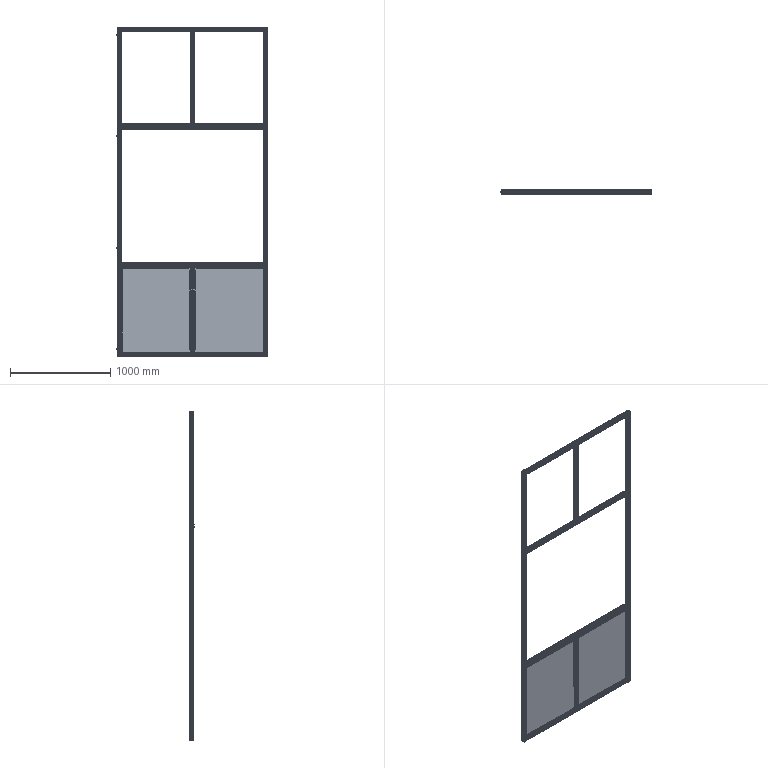Part | SolidWorks | features ReferencePattern 29, LocalLPattern 9 | 72 solids | 3442 faces | volume 15381691 mm3 | plane 2265 | cylinder 985 | cone 182 | spline 10 | commonest cylinder face diameters 6.8 x188 2 x102 19 x72 5 x66 8 x64 1 x48